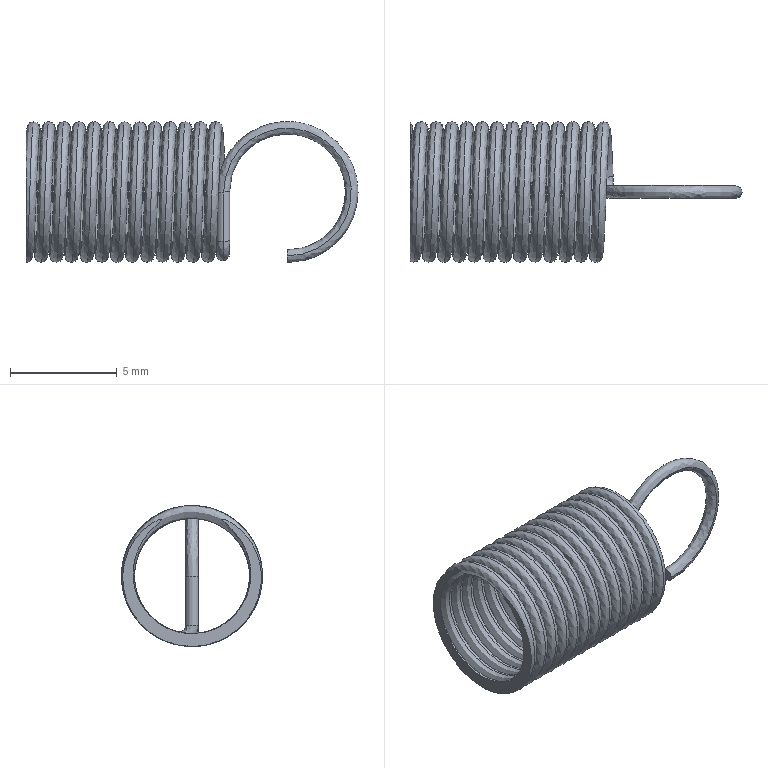Part | STEP file | 0246_011_AUY6-25 | 1 solid | 10 faces | volume 73.722 mm3 | spline 8 | plane 2